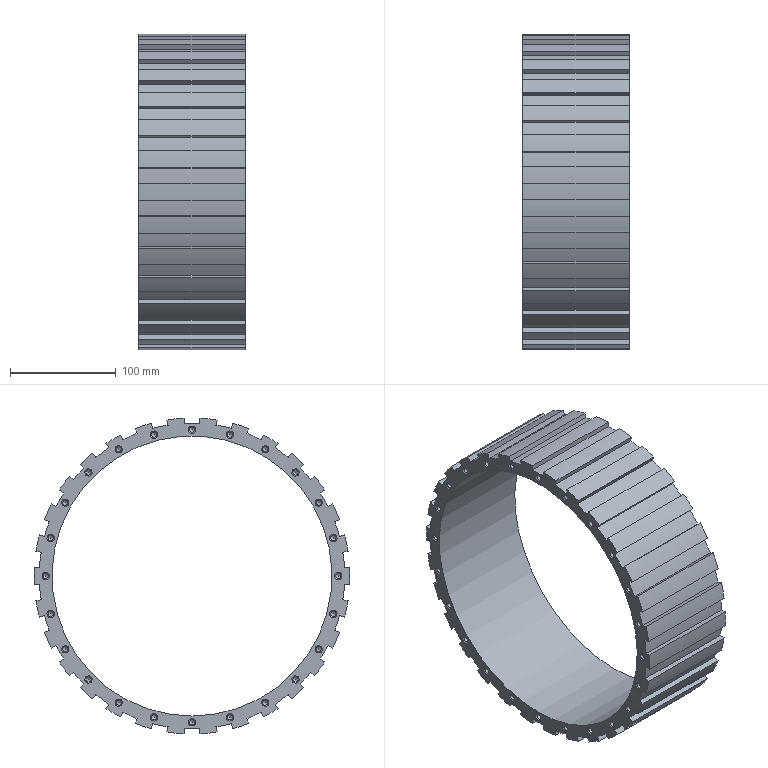Part | STEP file | Rotor | 1 solid | 267 faces | box 101 x 299 x 298.624 mm | volume 1274689 mm3 | cylinder 109 | cone 96 | plane 62 | commonest cylinder face diameters 4.917 x48 289 x30 299 x30 265 x1